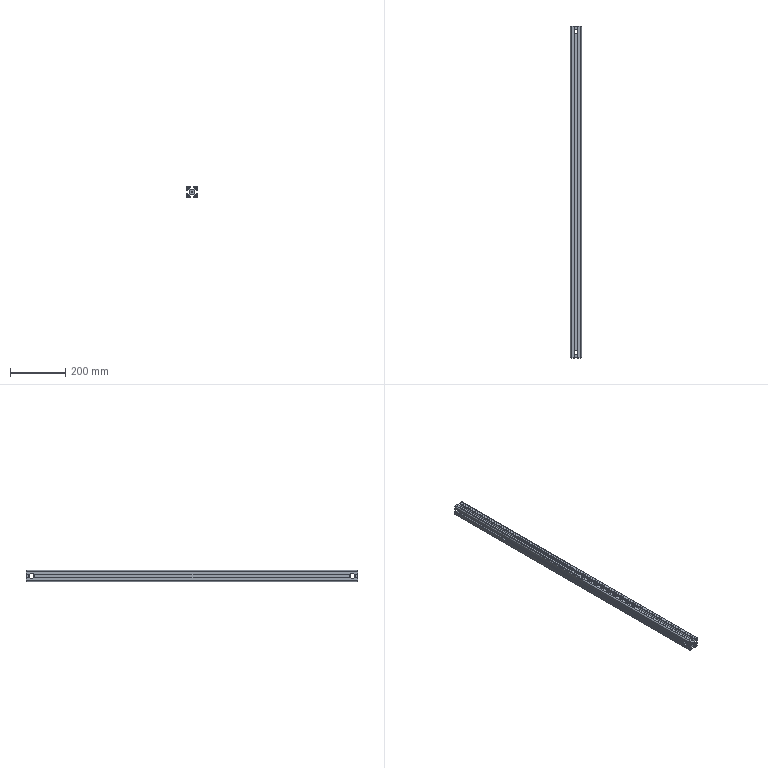Part | SolidWorks | features ICE 1, WeldMemberFeat 1, WeldmentFeature 1 | 1 solid | 160 faces | box 40 x 1203 x 40 mm | volume 719325 mm3 | plane 126 | cylinder 34 | commonest cylinder face diameters 19 x16 6 x8 6.8 x6 9 x4